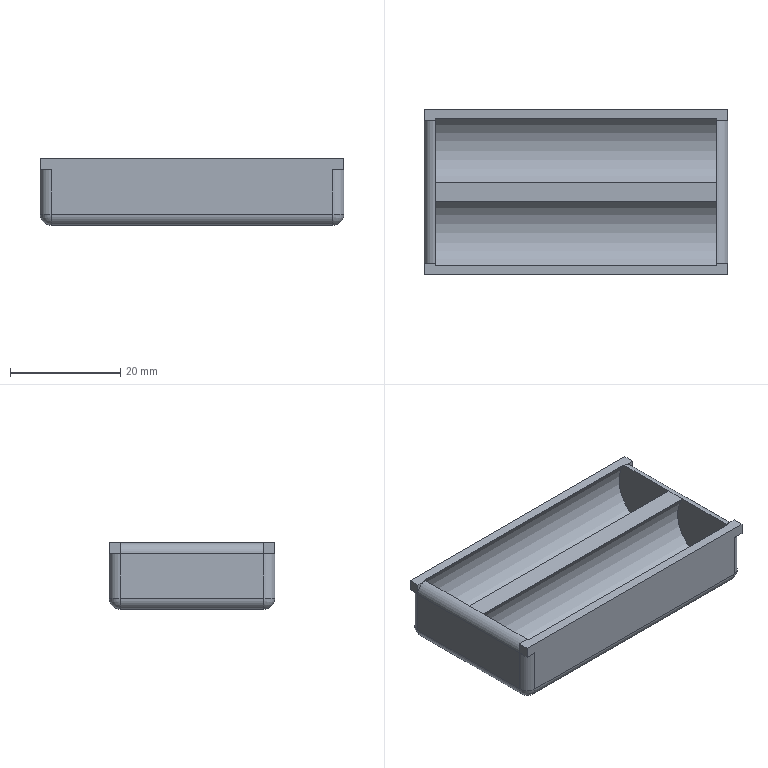Part | NX | features DATUM_CSYS 3, EXTRUDE 2, SKETCH 2, BLEND 1 | 1 solid | 40 faces | box 55 x 30 x 12 mm | volume 6346 mm3 | plane 24 | cylinder 12 | sphere 4 | commonest cylinder face diameters 4 x10 14 x2
STEP:
#1=CARTESIAN_POINT('',(-27.5,-13.,12.));
#2=VERTEX_POINT('',#1);
#3=CARTESIAN_POINT('',(-27.5,-15.,12.));
#4=VERTEX_POINT('',#3);
#5=CARTESIAN_POINT('',(-27.5,15.,12.));
#6=DIRECTION('',(0.,-1.,0.));
#7=VECTOR('',#6,1000.);
#8=LINE('',#5,#7);
#9=EDGE_CURVE('',#2,#4,#8,.T.);
#10=ORIENTED_EDGE('',*,*,#9,.F.);
#11=CARTESIAN_POINT('',(-27.5,-13.,10.));
#12=VERTEX_POINT('',#11);
#13=CARTESIAN_POINT('',(-27.5,-13.,12.));
#14=DIRECTION('',(0.,0.,-1.));
#15=VECTOR('',#14,1000.);
#16=LINE('',#13,#15);
#17=EDGE_CURVE('',#2,#12,#16,.T.);
#18=ORIENTED_EDGE('',*,*,#17,.T.);
#19=CARTESIAN_POINT('',(-27.5,-15.,10.));
#20=VERTEX_POINT('',#19);
#21=CARTESIAN_POINT('',(-27.5,-13.,10.));
#22=DIRECTION('',(0.,-1.,0.));
#23=VECTOR('',#22,1000.);
#24=LINE('',#21,#23);
#25=EDGE_CURVE('',#12,#20,#24,.T.);
#26=ORIENTED_EDGE('',*,*,#25,.T.);
#27=CARTESIAN_POINT('',(-27.5,-15.,12.));
#28=DIRECTION('',(0.,0.,-1.));
#29=VECTOR('',#28,1000.);
#30=LINE('',#27,#29);
#31=EDGE_CURVE('',#4,#20,#30,.T.);
#32=ORIENTED_EDGE('',*,*,#31,.F.);
#33=EDGE_LOOP('',(#10,#18,#26,#32));
#34=FACE_BOUND('',#33,.T.);
#35=CARTESIAN_POINT('',(-27.5,15.,12.));
#36=DIRECTION('',(1.,0.,0.));
#37=DIRECTION('',(0.,1.,0.));
#38=AXIS2_PLACEMENT_3D('',#35,#36,#37);
#39=PLANE('',#38);
#40=ADVANCED_FACE('',(#34),#39,.F.);
#41=CARTESIAN_POINT('',(-27.5,15.,10.));
#42=VERTEX_POINT('',#41);
#43=CARTESIAN_POINT('',(-27.5,13.,10.));
#44=VERTEX_POINT('',#43);
#45=CARTESIAN_POINT('',(-27.5,13.,10.));
#46=DIRECTION('',(0.,-1.,0.));
#47=VECTOR('',#46,1000.);
#48=LINE('',#45,#47);
#49=EDGE_CURVE('',#42,#44,#48,.T.);
#50=ORIENTED_EDGE('',*,*,#49,.T.);
#51=CARTESIAN_POINT('',(-27.5,13.,12.));
#52=VERTEX_POINT('',#51);
#53=CARTESIAN_POINT('',(-27.5,13.,12.));
#54=DIRECTION('',(0.,0.,1.));
#55=VECTOR('',#54,1000.);
#56=LINE('',#53,#55);
#57=EDGE_CURVE('',#44,#52,#56,.T.);
#58=ORIENTED_EDGE('',*,*,#57,.T.);
#59=CARTESIAN_POINT('',(-27.5,15.,12.));
#60=VERTEX_POINT('',#59);
#61=CARTESIAN_POINT('',(-27.5,15.,12.));
#62=DIRECTION('',(0.,-1.,0.));
#63=VECTOR('',#62,1000.);
#64=LINE('',#61,#63);
#65=EDGE_CURVE('',#60,#52,#64,.T.);
#66=ORIENTED_EDGE('',*,*,#65,.F.);
#67=CARTESIAN_POINT('',(-27.5,15.,12.));
#68=DIRECTION('',(0.,0.,-1.));
#69=VECTOR('',#68,1000.);
#70=LINE('',#67,#69);
#71=EDGE_CURVE('',#60,#42,#70,.T.);
#72=ORIENTED_EDGE('',*,*,#71,.T.);
#73=EDGE_LOOP('',(#50,#58,#66,#72));
#74=FACE_BOUND('',#73,.T.);
#75=CARTESIAN_POINT('',(-27.5,15.,12.));
#76=DIRECTION('',(1.,0.,0.));
#77=DIRECTION('',(0.,1.,0.));
#78=AXIS2_PLACEMENT_3D('',#75,#76,#77);
#79=PLANE('',#78);
#80=ADVANCED_FACE('',(#74),#79,.F.);
#81=CARTESIAN_POINT('',(27.5,13.,12.));
#82=VERTEX_POINT('',#81);
#83=CARTESIAN_POINT('',(27.5,15.,12.));
#84=VERTEX_POINT('',#83);
#85=CARTESIAN_POINT('',(27.5,-15.,12.));
#86=DIRECTION('',(0.,1.,0.));
#87=VECTOR('',#86,1000.);
#88=LINE('',#85,#87);
#89=EDGE_CURVE('',#82,#84,#88,.T.);
#90=ORIENTED_EDGE('',*,*,#89,.F.);
#91=CARTESIAN_POINT('',(27.5,13.,10.));
#92=VERTEX_POINT('',#91);
#93=CARTESIAN_POINT('',(27.5,13.,12.));
#94=DIRECTION('',(0.,0.,-1.));
#95=VECTOR('',#94,1000.);
#96=LINE('',#93,#95);
#97=EDGE_CURVE('',#82,#92,#96,.T.);
#98=ORIENTED_EDGE('',*,*,#97,.T.);
#99=CARTESIAN_POINT('',(27.5,15.,10.));
#100=VERTEX_POINT('',#99);
#101=CARTESIAN_POINT('',(27.5,13.,10.));
#102=DIRECTION('',(0.,1.,0.));
#103=VECTOR('',#102,1000.);
#104=LINE('',#101,#103);
#105=EDGE_CURVE('',#92,#100,#104,.T.);
#106=ORIENTED_EDGE('',*,*,#105,.T.);
#107=CARTESIAN_POINT('',(27.5,15.,12.));
#108=DIRECTION('',(0.,0.,-1.));
#109=VECTOR('',#108,1000.);
#110=LINE('',#107,#109);
#111=EDGE_CURVE('',#84,#100,#110,.T.);
#112=ORIENTED_EDGE('',*,*,#111,.F.);
#113=EDGE_LOOP('',(#90,#98,#106,#112));
#114=FACE_BOUND('',#113,.T.);
#115=CARTESIAN_POINT('',(27.5,-15.,12.));
#116=DIRECTION('',(-1.,0.,0.));
#117=DIRECTION('',(0.,-1.,0.));
#118=AXIS2_PLACEMENT_3D('',#115,#116,#117);
#119=PLANE('',#118);
#120=ADVANCED_FACE('',(#114),#119,.F.);
#121=CARTESIAN_POINT('',(27.5,-15.,10.));
#122=VERTEX_POINT('',#121);
#123=CARTESIAN_POINT('',(27.5,-13.,10.));
#124=VERTEX_POINT('',#123);
#125=CARTESIAN_POINT('',(27.5,-13.,10.));
#126=DIRECTION('',(0.,1.,0.));
#127=VECTOR('',#126,1000.);
#128=LINE('',#125,#127);
#129=EDGE_CURVE('',#122,#124,#128,.T.);
#130=ORIENTED_EDGE('',*,*,#129,.T.);
#131=CARTESIAN_POINT('',(27.5,-13.,12.));
#132=VERTEX_POINT('',#131);
#133=CARTESIAN_POINT('',(27.5,-13.,12.));
#134=DIRECTION('',(0.,0.,1.));
#135=VECTOR('',#134,1000.);
#136=LINE('',#133,#135);
#137=EDGE_CURVE('',#124,#132,#136,.T.);
#138=ORIENTED_EDGE('',*,*,#137,.T.);
#139=CARTESIAN_POINT('',(27.5,-15.,12.));
#140=VERTEX_POINT('',#139);
#141=CARTESIAN_POINT('',(27.5,-15.,12.));
#142=DIRECTION('',(0.,1.,0.));
#143=VECTOR('',#142,1000.);
#144=LINE('',#141,#143);
#145=EDGE_CURVE('',#140,#132,#144,.T.);
#146=ORIENTED_EDGE('',*,*,#145,.F.);
#147=CARTESIAN_POINT('',(27.5,-15.,12.));
#148=DIRECTION('',(0.,0.,-1.));
#149=VECTOR('',#148,1000.);
#150=LINE('',#147,#149);
#151=EDGE_CURVE('',#140,#122,#150,.T.);
#152=ORIENTED_EDGE('',*,*,#151,.T.);
#153=EDGE_LOOP('',(#130,#138,#146,#152));
#154=FACE_BOUND('',#153,.T.);
#155=CARTESIAN_POINT('',(27.5,-15.,12.));
#156=DIRECTION('',(-1.,0.,0.));
#157=DIRECTION('',(0.,-1.,0.));
#158=AXIS2_PLACEMENT_3D('',#155,#156,#157);
#159=PLANE('',#158);
#160=ADVANCED_FACE('',(#154),#159,.F.);
#161=ORIENTED_EDGE('',*,*,#145,.T.);
#162=CARTESIAN_POINT('',(25.5,-13.,12.));
#163=VERTEX_POINT('',#162);
#164=CARTESIAN_POINT('',(25.5,-13.,12.));
#165=DIRECTION('',(-1.,0.,0.));
#166=VECTOR('',#165,1000.);
#167=LINE('',#164,#166);
#168=EDGE_CURVE('',#132,#163,#167,.T.);
#169=ORIENTED_EDGE('',*,*,#168,.T.);
#170=CARTESIAN_POINT('',(25.5,-13.245,12.));
#171=VERTEX_POINT('',#170);
#172=CARTESIAN_POINT('',(25.5,0.,12.));
#173=DIRECTION('',(0.,-1.,0.));
#174=VECTOR('',#173,1000.);
#175=LINE('',#172,#174);
#176=EDGE_CURVE('',#163,#171,#175,.T.);
#177=ORIENTED_EDGE('',*,*,#176,.T.);
#178=CARTESIAN_POINT('',(-25.5,-13.245,12.));
#179=VERTEX_POINT('',#178);
#180=CARTESIAN_POINT('',(25.5,-13.245,12.));
#181=DIRECTION('',(-1.,0.,0.));
#182=VECTOR('',#181,1000.);
#183=LINE('',#180,#182);
#184=EDGE_CURVE('',#179,#171,#183,.F.);
#185=ORIENTED_EDGE('',*,*,#184,.F.);
#186=CARTESIAN_POINT('',(-25.5,-13.,12.));
#187=VERTEX_POINT('',#186);
#188=CARTESIAN_POINT('',(-25.5,0.,12.));
#189=DIRECTION('',(0.,-1.,0.));
#190=VECTOR('',#189,1000.);
#191=LINE('',#188,#190);
#192=EDGE_CURVE('',#187,#179,#191,.T.);
#193=ORIENTED_EDGE('',*,*,#192,.F.);
#194=CARTESIAN_POINT('',(-25.5,-13.,12.));
#195=DIRECTION('',(-1.,0.,0.));
#196=VECTOR('',#195,1000.);
#197=LINE('',#194,#196);
#198=EDGE_CURVE('',#187,#2,#197,.T.);
#199=ORIENTED_EDGE('',*,*,#198,.T.);
#200=ORIENTED_EDGE('',*,*,#9,.T.);
#201=CARTESIAN_POINT('',(-27.5,-15.,12.));
#202=DIRECTION('',(1.,0.,0.));
#203=VECTOR('',#202,1000.);
#204=LINE('',#201,#203);
#205=EDGE_CURVE('',#4,#140,#204,.T.);
#206=ORIENTED_EDGE('',*,*,#205,.T.);
#207=EDGE_LOOP('',(#161,#169,#177,#185,#193,#199,#200,#206));
#208=FACE_BOUND('',#207,.T.);
#209=CARTESIAN_POINT('',(0.,0.,12.));
#210=DIRECTION('',(0.,0.,1.));
#211=DIRECTION('',(1.,0.,0.));
#212=AXIS2_PLACEMENT_3D('',#209,#210,#211);
#213=PLANE('',#212);
#214=ADVANCED_FACE('',(#208),#213,.T.);
#215=CARTESIAN_POINT('',(25.5,-1.755,12.));
#216=VERTEX_POINT('',#215);
#217=CARTESIAN_POINT('',(-25.5,-1.755,12.));
#218=VERTEX_POINT('',#217);
#219=CARTESIAN_POINT('',(25.5,-1.755,12.));
#220=DIRECTION('',(-1.,0.,0.));
#221=VECTOR('',#220,1000.);
#222=LINE('',#219,#221);
#223=EDGE_CURVE('',#216,#218,#222,.T.);
#224=ORIENTED_EDGE('',*,*,#223,.F.);
#225=CARTESIAN_POINT('',(25.5,1.755,12.));
#226=VERTEX_POINT('',#225);
#227=CARTESIAN_POINT('',(25.5,15.,12.));
#228=DIRECTION('',(0.,1.,0.));
#229=VECTOR('',#228,1000.);
#230=LINE('',#227,#229);
#231=EDGE_CURVE('',#216,#226,#230,.T.);
#232=ORIENTED_EDGE('',*,*,#231,.T.);
#233=CARTESIAN_POINT('',(-25.5,1.755,12.));
#234=VERTEX_POINT('',#233);
#235=CARTESIAN_POINT('',(25.5,1.755,12.));
#236=DIRECTION('',(-1.,0.,0.));
#237=VECTOR('',#236,1000.);
#238=LINE('',#235,#237);
#239=EDGE_CURVE('',#234,#226,#238,.F.);
#240=ORIENTED_EDGE('',*,*,#239,.F.);
#241=CARTESIAN_POINT('',(-25.5,-15.,12.));
#242=DIRECTION('',(0.,-1.,0.));
#243=VECTOR('',#242,1000.);
#244=LINE('',#241,#243);
#245=EDGE_CURVE('',#234,#218,#244,.T.);
#246=ORIENTED_EDGE('',*,*,#245,.T.);
#247=EDGE_LOOP('',(#224,#232,#240,#246));
#248=FACE_BOUND('',#247,.T.);
#249=CARTESIAN_POINT('',(0.,0.,12.));
#250=DIRECTION('',(0.,0.,1.));
#251=DIRECTION('',(1.,0.,0.));
#252=AXIS2_PLACEMENT_3D('',#249,#250,#251);
#253=PLANE('',#252);
#254=ADVANCED_FACE('',(#248),#253,.T.);
#255=CARTESIAN_POINT('',(25.5,13.245,12.));
#256=VERTEX_POINT('',#255);
#257=CARTESIAN_POINT('',(25.5,13.,12.));
#258=VERTEX_POINT('',#257);
#259=CARTESIAN_POINT('',(25.5,0.,12.));
#260=DIRECTION('',(0.,-1.,0.));
#261=VECTOR('',#260,1000.);
#262=LINE('',#259,#261);
#263=EDGE_CURVE('',#256,#258,#262,.T.);
#264=ORIENTED_EDGE('',*,*,#263,.T.);
#265=CARTESIAN_POINT('',(25.5,13.,12.));
#266=DIRECTION('',(1.,0.,0.));
#267=VECTOR('',#266,1000.);
#268=LINE('',#265,#267);
#269=EDGE_CURVE('',#258,#82,#268,.T.);
#270=ORIENTED_EDGE('',*,*,#269,.T.);
#271=ORIENTED_EDGE('',*,*,#89,.T.);
#272=CARTESIAN_POINT('',(27.5,15.,12.));
#273=DIRECTION('',(-1.,0.,0.));
#274=VECTOR('',#273,1000.);
#275=LINE('',#272,#274);
#276=EDGE_CURVE('',#84,#60,#275,.T.);
#277=ORIENTED_EDGE('',*,*,#276,.T.);
#278=ORIENTED_EDGE('',*,*,#65,.T.);
#279=CARTESIAN_POINT('',(-25.5,13.,12.));
#280=VERTEX_POINT('',#279);
#281=CARTESIAN_POINT('',(-25.5,13.,12.));
#282=DIRECTION('',(1.,0.,0.));
#283=VECTOR('',#282,1000.);
#284=LINE('',#281,#283);
#285=EDGE_CURVE('',#52,#280,#284,.T.);
#286=ORIENTED_EDGE('',*,*,#285,.T.);
#287=CARTESIAN_POINT('',(-25.5,13.245,12.));
#288=VERTEX_POINT('',#287);
#289=CARTESIAN_POINT('',(-25.5,0.,12.));
#290=DIRECTION('',(0.,-1.,0.));
#291=VECTOR('',#290,1000.);
#292=LINE('',#289,#291);
#293=EDGE_CURVE('',#288,#280,#292,.T.);
#294=ORIENTED_EDGE('',*,*,#293,.F.);
#295=CARTESIAN_POINT('',(25.5,13.245,12.));
#296=DIRECTION('',(-1.,0.,0.));
#297=VECTOR('',#296,1000.);
#298=LINE('',#295,#297);
#299=EDGE_CURVE('',#256,#288,#298,.T.);
#300=ORIENTED_EDGE('',*,*,#299,.F.);
#301=EDGE_LOOP('',(#264,#270,#271,#277,#278,#286,#294,#300));
#302=FACE_BOUND('',#301,.T.);
#303=CARTESIAN_POINT('',(0.,0.,12.));
#304=DIRECTION('',(0.,0.,1.));
#305=DIRECTION('',(1.,0.,0.));
#306=AXIS2_PLACEMENT_3D('',#303,#304,#305);
#307=PLANE('',#306);
#308=ADVANCED_FACE('',(#302),#307,.T.);
#309=CARTESIAN_POINT('',(-27.5,-13.,2.));
#310=VERTEX_POINT('',#309);
#311=CARTESIAN_POINT('',(-27.5,-13.,12.));
#312=DIRECTION('',(0.,0.,-1.));
#313=VECTOR('',#312,1000.);
#314=LINE('',#311,#313);
#315=EDGE_CURVE('',#310,#12,#314,.F.);
#316=ORIENTED_EDGE('',*,*,#315,.T.);
#317=CARTESIAN_POINT('',(-27.5,15.,10.));
#318=DIRECTION('',(0.,-1.,0.));
#319=VECTOR('',#318,1000.);
#320=LINE('',#317,#319);
#321=EDGE_CURVE('',#12,#44,#320,.F.);
#322=ORIENTED_EDGE('',*,*,#321,.T.);
#323=CARTESIAN_POINT('',(-27.5,13.,2.));
#324=VERTEX_POINT('',#323);
#325=CARTESIAN_POINT('',(-27.5,13.,12.));
#326=DIRECTION('',(0.,0.,-1.));
#327=VECTOR('',#326,1000.);
#328=LINE('',#325,#327);
#329=EDGE_CURVE('',#44,#324,#328,.T.);
#330=ORIENTED_EDGE('',*,*,#329,.T.);
#331=CARTESIAN_POINT('',(-27.5,15.,2.));
#332=DIRECTION('',(0.,-1.,0.));
#333=VECTOR('',#332,1000.);
#334=LINE('',#331,#333);
#335=EDGE_CURVE('',#324,#310,#334,.T.);
#336=ORIENTED_EDGE('',*,*,#335,.T.);
#337=EDGE_LOOP('',(#316,#322,#330,#336));
#338=FACE_BOUND('',#337,.T.);
#339=CARTESIAN_POINT('',(-27.5,15.,12.));
#340=DIRECTION('',(1.,0.,0.));
#341=DIRECTION('',(0.,1.,0.));
#342=AXIS2_PLACEMENT_3D('',#339,#340,#341);
#343=PLANE('',#342);
#344=ADVANCED_FACE('',(#338),#343,.F.);
#345=CARTESIAN_POINT('',(25.5,-15.,2.));
#346=VERTEX_POINT('',#345);
#347=CARTESIAN_POINT('',(25.5,-15.,10.));
#348=VERTEX_POINT('',#347);
#349=CARTESIAN_POINT('',(25.5,-15.,12.));
#350=DIRECTION('',(0.,0.,-1.));
#351=VECTOR('',#350,1000.);
#352=LINE('',#349,#351);
#353=EDGE_CURVE('',#346,#348,#352,.F.);
#354=ORIENTED_EDGE('',*,*,#353,.T.);
#355=CARTESIAN_POINT('',(25.5,-15.,10.));
#356=DIRECTION('',(1.,0.,0.));
#357=VECTOR('',#356,1000.);
#358=LINE('',#355,#357);
#359=EDGE_CURVE('',#348,#122,#358,.T.);
#360=ORIENTED_EDGE('',*,*,#359,.T.);
#361=ORIENTED_EDGE('',*,*,#151,.F.);
#362=ORIENTED_EDGE('',*,*,#205,.F.);
#363=ORIENTED_EDGE('',*,*,#31,.T.);
#364=CARTESIAN_POINT('',(-25.5,-15.,10.));
#365=VERTEX_POINT('',#364);
#366=CARTESIAN_POINT('',(-25.5,-15.,10.));
#367=DIRECTION('',(1.,0.,0.));
#368=VECTOR('',#367,1000.);
#369=LINE('',#366,#368);
#370=EDGE_CURVE('',#20,#365,#369,.T.);
#371=ORIENTED_EDGE('',*,*,#370,.T.);
#372=CARTESIAN_POINT('',(-25.5,-15.,2.));
#373=VERTEX_POINT('',#372);
#374=CARTESIAN_POINT('',(-25.5,-15.,12.));
#375=DIRECTION('',(0.,0.,-1.));
#376=VECTOR('',#375,1000.);
#377=LINE('',#374,#376);
#378=EDGE_CURVE('',#365,#373,#377,.T.);
#379=ORIENTED_EDGE('',*,*,#378,.T.);
#380=CARTESIAN_POINT('',(-27.5,-15.,2.));
#381=DIRECTION('',(1.,0.,0.));
#382=VECTOR('',#381,1000.);
#383=LINE('',#380,#382);
#384=EDGE_CURVE('',#373,#346,#383,.T.);
#385=ORIENTED_EDGE('',*,*,#384,.T.);
#386=EDGE_LOOP('',(#354,#360,#361,#362,#363,#371,#379,#385));
#387=FACE_BOUND('',#386,.T.);
#388=CARTESIAN_POINT('',(-27.5,-15.,12.));
#389=DIRECTION('',(0.,1.,0.));
#390=DIRECTION('',(0.,0.,1.));
#391=AXIS2_PLACEMENT_3D('',#388,#389,#390);
#392=PLANE('',#391);
#393=ADVANCED_FACE('',(#387),#392,.F.);
#394=CARTESIAN_POINT('',(27.5,13.,2.));
#395=VERTEX_POINT('',#394);
#396=CARTESIAN_POINT('',(27.5,13.,12.));
#397=DIRECTION('',(0.,0.,-1.));
#398=VECTOR('',#397,1000.);
#399=LINE('',#396,#398);
#400=EDGE_CURVE('',#395,#92,#399,.F.);
#401=ORIENTED_EDGE('',*,*,#400,.T.);
#402=CARTESIAN_POINT('',(27.5,-15.,10.));
#403=DIRECTION('',(0.,1.,0.));
#404=VECTOR('',#403,1000.);
#405=LINE('',#402,#404);
#406=EDGE_CURVE('',#92,#124,#405,.F.);
#407=ORIENTED_EDGE('',*,*,#406,.T.);
#408=CARTESIAN_POINT('',(27.5,-13.,2.));
#409=VERTEX_POINT('',#408);
#410=CARTESIAN_POINT('',(27.5,-13.,12.));
#411=DIRECTION('',(0.,0.,-1.));
#412=VECTOR('',#411,1000.);
#413=LINE('',#410,#412);
#414=EDGE_CURVE('',#124,#409,#413,.T.);
#415=ORIENTED_EDGE('',*,*,#414,.T.);
#416=CARTESIAN_POINT('',(27.5,-15.,2.));
#417=DIRECTION('',(0.,1.,0.));
#418=VECTOR('',#417,1000.);
#419=LINE('',#416,#418);
#420=EDGE_CURVE('',#409,#395,#419,.T.);
#421=ORIENTED_EDGE('',*,*,#420,.T.);
#422=EDGE_LOOP('',(#401,#407,#415,#421));
#423=FACE_BOUND('',#422,.T.);
#424=CARTESIAN_POINT('',(27.5,-15.,12.));
#425=DIRECTION('',(-1.,0.,0.));
#426=DIRECTION('',(0.,-1.,0.));
#427=AXIS2_PLACEMENT_3D('',#424,#425,#426);
#428=PLANE('',#427);
#429=ADVANCED_FACE('',(#423),#428,.F.);
#430=ORIENTED_EDGE('',*,*,#111,.T.);
#431=CARTESIAN_POINT('',(25.5,15.,10.));
#432=VERTEX_POINT('',#431);
#433=CARTESIAN_POINT('',(25.5,15.,10.));
#434=DIRECTION('',(-1.,0.,0.));
#435=VECTOR('',#434,1000.);
#436=LINE('',#433,#435);
#437=EDGE_CURVE('',#100,#432,#436,.T.);
#438=ORIENTED_EDGE('',*,*,#437,.T.);
#439=CARTESIAN_POINT('',(25.5,15.,2.));
#440=VERTEX_POINT('',#439);
#441=CARTESIAN_POINT('',(25.5,15.,12.));
#442=DIRECTION('',(0.,0.,-1.));
#443=VECTOR('',#442,1000.);
#444=LINE('',#441,#443);
#445=EDGE_CURVE('',#432,#440,#444,.T.);
#446=ORIENTED_EDGE('',*,*,#445,.T.);
#447=CARTESIAN_POINT('',(-25.5,15.,2.));
#448=VERTEX_POINT('',#447);
#449=CARTESIAN_POINT('',(27.5,15.,2.));
#450=DIRECTION('',(-1.,0.,0.));
#451=VECTOR('',#450,1000.);
#452=LINE('',#449,#451);
#453=EDGE_CURVE('',#440,#448,#452,.T.);
#454=ORIENTED_EDGE('',*,*,#453,.T.);
#455=CARTESIAN_POINT('',(-25.5,15.,10.));
#456=VERTEX_POINT('',#455);
#457=CARTESIAN_POINT('',(-25.5,15.,12.));
#458=DIRECTION('',(0.,0.,-1.));
#459=VECTOR('',#458,1000.);
#460=LINE('',#457,#459);
#461=EDGE_CURVE('',#448,#456,#460,.F.);
#462=ORIENTED_EDGE('',*,*,#461,.T.);
#463=CARTESIAN_POINT('',(-25.5,15.,10.));
#464=DIRECTION('',(-1.,0.,0.));
#465=VECTOR('',#464,1000.);
#466=LINE('',#463,#465);
#467=EDGE_CURVE('',#456,#42,#466,.T.);
#468=ORIENTED_EDGE('',*,*,#467,.T.);
#469=ORIENTED_EDGE('',*,*,#71,.F.);
#470=ORIENTED_EDGE('',*,*,#276,.F.);
#471=EDGE_LOOP('',(#430,#438,#446,#454,#462,#468,#469,#470));
#472=FACE_BOUND('',#471,.T.);
#473=CARTESIAN_POINT('',(27.5,15.,12.));
#474=DIRECTION('',(0.,-1.,0.));
#475=DIRECTION('',(1.,0.,0.));
#476=AXIS2_PLACEMENT_3D('',#473,#474,#475);
#477=PLANE('',#476);
#478=ADVANCED_FACE('',(#472),#477,.F.);
#479=CARTESIAN_POINT('',(25.5,-13.,0.));
#480=VERTEX_POINT('',#479);
#481=CARTESIAN_POINT('',(-25.5,-13.,0.));
#482=VERTEX_POINT('',#481);
#483=CARTESIAN_POINT('',(0.,-13.,0.));
#484=DIRECTION('',(1.,0.,0.));
#485=VECTOR('',#484,1000.);
#486=LINE('',#483,#485);
#487=EDGE_CURVE('',#480,#482,#486,.F.);
#488=ORIENTED_EDGE('',*,*,#487,.T.);
#489=CARTESIAN_POINT('',(-25.5,13.,0.));
#490=VERTEX_POINT('',#489);
#491=CARTESIAN_POINT('',(-25.5,0.,0.));
#492=DIRECTION('',(0.,-1.,0.));
#493=VECTOR('',#492,1000.);
#494=LINE('',#491,#493);
#495=EDGE_CURVE('',#482,#490,#494,.F.);
#496=ORIENTED_EDGE('',*,*,#495,.T.);
#497=CARTESIAN_POINT('',(25.5,13.,0.));
#498=VERTEX_POINT('',#497);
#499=CARTESIAN_POINT('',(0.,13.,0.));
#500=DIRECTION('',(-1.,0.,0.));
#501=VECTOR('',#500,1000.);
#502=LINE('',#499,#501);
#503=EDGE_CURVE('',#490,#498,#502,.F.);
#504=ORIENTED_EDGE('',*,*,#503,.T.);
#505=CARTESIAN_POINT('',(25.5,0.,0.));
#506=DIRECTION('',(0.,1.,0.));
#507=VECTOR('',#506,1000.);
#508=LINE('',#505,#507);
#509=EDGE_CURVE('',#498,#480,#508,.F.);
#510=ORIENTED_EDGE('',*,*,#509,.T.);
#511=EDGE_LOOP('',(#488,#496,#504,#510));
#512=FACE_BOUND('',#511,.T.);
#513=CARTESIAN_POINT('',(0.,0.,0.));
#514=DIRECTION('',(0.,0.,1.));
#515=DIRECTION('',(1.,0.,0.));
#516=AXIS2_PLACEMENT_3D('',#513,#514,#515);
#517=PLANE('',#516);
#518=ADVANCED_FACE('',(#512),#517,.F.);
#519=ORIENTED_EDGE('',*,*,#299,.T.);
#520=CARTESIAN_POINT('',(-25.5,7.5,8.));
#521=DIRECTION('',(-1.,0.,0.));
#522=DIRECTION('',(0.,1.,0.));
#523=AXIS2_PLACEMENT_3D('',#520,#521,#522);
#524=CIRCLE('',#523,7.);
#525=EDGE_CURVE('',#234,#288,#524,.F.);
#526=ORIENTED_EDGE('',*,*,#525,.F.);
#527=ORIENTED_EDGE('',*,*,#239,.T.);
#528=CARTESIAN_POINT('',(25.5,7.5,8.));
#529=DIRECTION('',(-1.,0.,0.));
#530=DIRECTION('',(0.,1.,0.));
#531=AXIS2_PLACEMENT_3D('',#528,#529,#530);
#532=CIRCLE('',#531,7.);
#533=EDGE_CURVE('',#226,#256,#532,.F.);
#534=ORIENTED_EDGE('',*,*,#533,.T.);
#535=EDGE_LOOP('',(#519,#526,#527,#534));
#536=FACE_BOUND('',#535,.T.);
#537=CARTESIAN_POINT('',(25.5,7.5,8.));
#538=DIRECTION('',(-1.,0.,0.));
#539=DIRECTION('',(0.,0.,1.));
#540=AXIS2_PLACEMENT_3D('',#537,#538,#539);
#541=CYLINDRICAL_SURFACE('',#540,7.);
#542=ADVANCED_FACE('',(#536),#541,.F.);
#543=ORIENTED_EDGE('',*,*,#533,.F.);
#544=CARTESIAN_POINT('',(25.5,0.,12.));
#545=DIRECTION('',(0.,-1.,0.));
#546=VECTOR('',#545,1000.);
#547=LINE('',#544,#546);
#548=EDGE_CURVE('',#258,#226,#547,.T.);
#549=ORIENTED_EDGE('',*,*,#548,.F.);
#550=ORIENTED_EDGE('',*,*,#263,.F.);
#551=EDGE_LOOP('',(#543,#549,#550));
#552=FACE_BOUND('',#551,.T.);
#553=CARTESIAN_POINT('',(25.5,7.5,8.));
#554=DIRECTION('',(-1.,0.,0.));
#555=DIRECTION('',(0.,0.,1.));
#556=AXIS2_PLACEMENT_3D('',#553,#554,#555);
#557=PLANE('',#556);
#558=ADVANCED_FACE('',(#552),#557,.T.);
#559=ORIENTED_EDGE('',*,*,#293,.T.);
#560=CARTESIAN_POINT('',(-25.5,0.,12.));
#561=DIRECTION('',(0.,-1.,0.));
#562=VECTOR('',#561,1000.);
#563=LINE('',#560,#562);
#564=EDGE_CURVE('',#280,#234,#563,.T.);
#565=ORIENTED_EDGE('',*,*,#564,.T.);
#566=ORIENTED_EDGE('',*,*,#525,.T.);
#567=EDGE_LOOP('',(#559,#565,#566));
#568=FACE_BOUND('',#567,.T.);
#569=CARTESIAN_POINT('',(-25.5,7.5,8.));
#570=DIRECTION('',(-1.,0.,0.));
#571=DIRECTION('',(0.,0.,1.));
#572=AXIS2_PLACEMENT_3D('',#569,#570,#571);
#573=PLANE('',#572);
#574=ADVANCED_FACE('',(#568),#573,.F.);
#575=ORIENTED_EDGE('',*,*,#223,.T.);
#576=CARTESIAN_POINT('',(-25.5,-7.5,8.));
#577=DIRECTION('',(-1.,0.,0.));
#578=DIRECTION('',(0.,1.,0.));
#579=AXIS2_PLACEMENT_3D('',#576,#577,#578);
#580=CIRCLE('',#579,7.);
#581=EDGE_CURVE('',#179,#218,#580,.F.);
#582=ORIENTED_EDGE('',*,*,#581,.F.);
#583=ORIENTED_EDGE('',*,*,#184,.T.);
#584=CARTESIAN_POINT('',(25.5,-7.5,8.));
#585=DIRECTION('',(-1.,0.,0.));
#586=DIRECTION('',(0.,1.,0.));
#587=AXIS2_PLACEMENT_3D('',#584,#585,#586);
#588=CIRCLE('',#587,7.);
#589=EDGE_CURVE('',#171,#216,#588,.F.);
#590=ORIENTED_EDGE('',*,*,#589,.T.);
#591=EDGE_LOOP('',(#575,#582,#583,#590));
#592=FACE_BOUND('',#591,.T.);
#593=CARTESIAN_POINT('',(25.5,-7.5,8.));
#594=DIRECTION('',(-1.,0.,0.));
#595=DIRECTION('',(0.,0.,1.));
#596=AXIS2_PLACEMENT_3D('',#593,#594,#595);
#597=CYLINDRICAL_SURFACE('',#596,7.);
#598=ADVANCED_FACE('',(#592),#597,.F.);
#599=ORIENTED_EDGE('',*,*,#589,.F.);
#600=ORIENTED_EDGE('',*,*,#176,.F.);
#601=CARTESIAN_POINT('',(25.5,0.,12.));
#602=DIRECTION('',(0.,-1.,0.));
#603=VECTOR('',#602,1000.);
#604=LINE('',#601,#603);
#605=EDGE_CURVE('',#216,#163,#604,.T.);
#606=ORIENTED_EDGE('',*,*,#605,.F.);
#607=EDGE_LOOP('',(#599,#600,#606));
#608=FACE_BOUND('',#607,.T.);
#609=CARTESIAN_POINT('',(25.5,-7.5,8.));
#610=DIRECTION('',(-1.,0.,0.));
#611=DIRECTION('',(0.,0.,1.));
#612=AXIS2_PLACEMENT_3D('',#609,#610,#611);
#613=PLANE('',#612);
#614=ADVANCED_FACE('',(#608),#613,.T.);
#615=CARTESIAN_POINT('',(-25.5,0.,12.));
#616=DIRECTION('',(0.,-1.,0.));
#617=VECTOR('',#616,1000.);
#618=LINE('',#615,#617);
#619=EDGE_CURVE('',#218,#187,#618,.T.);
#620=ORIENTED_EDGE('',*,*,#619,.T.);
#621=ORIENTED_EDGE('',*,*,#192,.T.);
#622=ORIENTED_EDGE('',*,*,#581,.T.);
#623=EDGE_LOOP('',(#620,#621,#622));
#624=FACE_BOUND('',#623,.T.);
#625=CARTESIAN_POINT('',(-25.5,-7.5,8.));
#626=DIRECTION('',(-1.,0.,0.));
#627=DIRECTION('',(0.,0.,1.));
#628=AXIS2_PLACEMENT_3D('',#625,#626,#627);
#629=PLANE('',#628);
#630=ADVANCED_FACE('',(#624),#629,.F.);
#631=ORIENTED_EDGE('',*,*,#437,.F.);
#632=ORIENTED_EDGE('',*,*,#105,.F.);
#633=CARTESIAN_POINT('',(25.5,13.,10.));
#634=DIRECTION('',(0.,0.,1.));
#635=DIRECTION('',(1.,0.,0.));
#636=AXIS2_PLACEMENT_3D('',#633,#634,#635);
#637=CIRCLE('',#636,2.);
#638=EDGE_CURVE('',#432,#92,#637,.F.);
#639=ORIENTED_EDGE('',*,*,#638,.F.);
#640=EDGE_LOOP('',(#631,#632,#639));
#641=FACE_BOUND('',#640,.T.);
#642=CARTESIAN_POINT('',(25.5,13.,10.));
#643=DIRECTION('',(0.,0.,-1.));
#644=DIRECTION('',(-1.,0.,0.));
#645=AXIS2_PLACEMENT_3D('',#642,#643,#644);
#646=PLANE('',#645);
#647=ADVANCED_FACE('',(#641),#646,.T.);
#648=ORIENTED_EDGE('',*,*,#129,.F.);
#649=ORIENTED_EDGE('',*,*,#359,.F.);
#650=CARTESIAN_POINT('',(25.5,-13.,10.));
#651=DIRECTION('',(0.,0.,1.));
#652=DIRECTION('',(1.,0.,0.));
#653=AXIS2_PLACEMENT_3D('',#650,#651,#652);
#654=CIRCLE('',#653,2.);
#655=EDGE_CURVE('',#124,#348,#654,.F.);
#656=ORIENTED_EDGE('',*,*,#655,.F.);
#657=EDGE_LOOP('',(#648,#649,#656));
#658=FACE_BOUND('',#657,.T.);
#659=CARTESIAN_POINT('',(25.5,-13.,10.));
#660=DIRECTION('',(0.,0.,-1.));
#661=DIRECTION('',(-1.,0.,0.));
#662=AXIS2_PLACEMENT_3D('',#659,#660,#661);
#663=PLANE('',#662);
#664=ADVANCED_FACE('',(#658),#663,.T.);
#665=ORIENTED_EDGE('',*,*,#638,.T.);
#666=ORIENTED_EDGE('',*,*,#400,.F.);
#667=CARTESIAN_POINT('',(25.5,13.,2.));
#668=DIRECTION('',(0.,0.,-1.));
#669=DIRECTION('',(-1.,0.,0.));
#670=AXIS2_PLACEMENT_3D('',#667,#668,#669);
#671=CIRCLE('',#670,2.);
#672=EDGE_CURVE('',#440,#395,#671,.T.);
#673=ORIENTED_EDGE('',*,*,#672,.F.);
#674=ORIENTED_EDGE('',*,*,#445,.F.);
#675=EDGE_LOOP('',(#665,#666,#673,#674));
#676=FACE_BOUND('',#675,.T.);
#677=CARTESIAN_POINT('',(25.5,13.,12.));
#678=DIRECTION('',(0.,0.,-1.));
#679=DIRECTION('',(-1.,0.,0.));
#680=AXIS2_PLACEMENT_3D('',#677,#678,#679);
#681=CYLINDRICAL_SURFACE('',#680,2.);
#682=ADVANCED_FACE('',(#676),#681,.T.);
#683=ORIENTED_EDGE('',*,*,#655,.T.);
#684=ORIENTED_EDGE('',*,*,#353,.F.);
#685=CARTESIAN_POINT('',(25.5,-13.,2.));
#686=DIRECTION('',(0.,0.,-1.));
#687=DIRECTION('',(-1.,0.,0.));
#688=AXIS2_PLACEMENT_3D('',#685,#686,#687);
#689=CIRCLE('',#688,2.);
#690=EDGE_CURVE('',#409,#346,#689,.T.);
#691=ORIENTED_EDGE('',*,*,#690,.F.);
#692=ORIENTED_EDGE('',*,*,#414,.F.);
#693=EDGE_LOOP('',(#683,#684,#691,#692));
#694=FACE_BOUND('',#693,.T.);
#695=CARTESIAN_POINT('',(25.5,-13.,12.));
#696=DIRECTION('',(0.,0.,-1.));
#697=DIRECTION('',(-1.,0.,0.));
#698=AXIS2_PLACEMENT_3D('',#695,#696,#697);
#699=CYLINDRICAL_SURFACE('',#698,2.);
#700=ADVANCED_FACE('',(#694),#699,.T.);
#701=CARTESIAN_POINT('',(25.5,13.,2.));
#702=DIRECTION('',(0.,1.,0.));
#703=DIRECTION('',(0.,0.,1.));
#704=AXIS2_PLACEMENT_3D('',#701,#702,#703);
#705=CIRCLE('',#704,2.);
#706=EDGE_CURVE('',#395,#498,#705,.T.);
#707=ORIENTED_EDGE('',*,*,#706,.F.);
#708=ORIENTED_EDGE('',*,*,#420,.F.);
#709=CARTESIAN_POINT('',(25.5,-13.,2.));
#710=DIRECTION('',(0.,-1.,0.));
#711=DIRECTION('',(0.,0.,-1.));
#712=AXIS2_PLACEMENT_3D('',#709,#710,#711);
#713=CIRCLE('',#712,2.);
#714=EDGE_CURVE('',#480,#409,#713,.T.);
#715=ORIENTED_EDGE('',*,*,#714,.F.);
#716=ORIENTED_EDGE('',*,*,#509,.F.);
#717=EDGE_LOOP('',(#707,#708,#715,#716));
#718=FACE_BOUND('',#717,.T.);
#719=CARTESIAN_POINT('',(25.5,-15.,2.));
#720=DIRECTION('',(0.,1.,0.));
#721=DIRECTION('',(-1.,0.,0.));
#722=AXIS2_PLACEMENT_3D('',#719,#720,#721);
#723=CYLINDRICAL_SURFACE('',#722,2.);
#724=ADVANCED_FACE('',(#718),#723,.T.);
#725=ORIENTED_EDGE('',*,*,#672,.T.);
#726=ORIENTED_EDGE('',*,*,#706,.T.);
#727=CARTESIAN_POINT('',(25.5,13.,2.));
#728=DIRECTION('',(1.,0.,0.));
#729=DIRECTION('',(0.,0.,-1.));
#730=AXIS2_PLACEMENT_3D('',#727,#728,#729);
#731=CIRCLE('',#730,2.);
#732=EDGE_CURVE('',#440,#498,#731,.F.);
#733=ORIENTED_EDGE('',*,*,#732,.F.);
#734=EDGE_LOOP('',(#725,#726,#733));
#735=FACE_BOUND('',#734,.T.);
#736=CARTESIAN_POINT('',(25.5,13.,2.));
#737=DIRECTION('',(0.,0.,1.));
#738=DIRECTION('',(1.,0.,0.));
#739=AXIS2_PLACEMENT_3D('',#736,#737,#738);
#740=SPHERICAL_SURFACE('',#739,2.);
#741=ADVANCED_FACE('',(#735),#740,.T.);
#742=ORIENTED_EDGE('',*,*,#49,.F.);
#743=ORIENTED_EDGE('',*,*,#467,.F.);
#744=CARTESIAN_POINT('',(-25.5,13.,10.));
#745=DIRECTION('',(0.,0.,1.));
#746=DIRECTION('',(1.,0.,0.));
#747=AXIS2_PLACEMENT_3D('',#744,#745,#746);
#748=CIRCLE('',#747,2.);
#749=EDGE_CURVE('',#44,#456,#748,.F.);
#750=ORIENTED_EDGE('',*,*,#749,.F.);
#751=EDGE_LOOP('',(#742,#743,#750));
#752=FACE_BOUND('',#751,.T.);
#753=CARTESIAN_POINT('',(-25.5,13.,10.));
#754=DIRECTION('',(0.,0.,-1.));
#755=DIRECTION('',(-1.,0.,0.));
#756=AXIS2_PLACEMENT_3D('',#753,#754,#755);
#757=PLANE('',#756);
#758=ADVANCED_FACE('',(#752),#757,.T.);
#759=ORIENTED_EDGE('',*,*,#370,.F.);
#760=ORIENTED_EDGE('',*,*,#25,.F.);
#761=CARTESIAN_POINT('',(-25.5,-13.,10.));
#762=DIRECTION('',(0.,0.,1.));
#763=DIRECTION('',(1.,0.,0.));
#764=AXIS2_PLACEMENT_3D('',#761,#762,#763);
#765=CIRCLE('',#764,2.);
#766=EDGE_CURVE('',#365,#12,#765,.F.);
#767=ORIENTED_EDGE('',*,*,#766,.F.);
#768=EDGE_LOOP('',(#759,#760,#767));
#769=FACE_BOUND('',#768,.T.);
#770=CARTESIAN_POINT('',(-25.5,-13.,10.));
#771=DIRECTION('',(0.,0.,-1.));
#772=DIRECTION('',(-1.,0.,0.));
#773=AXIS2_PLACEMENT_3D('',#770,#771,#772);
#774=PLANE('',#773);
#775=ADVANCED_FACE('',(#769),#774,.T.);
#776=ORIENTED_EDGE('',*,*,#714,.T.);
#777=ORIENTED_EDGE('',*,*,#690,.T.);
#778=CARTESIAN_POINT('',(25.5,-13.,2.));
#779=DIRECTION('',(1.,0.,0.));
#780=DIRECTION('',(0.,0.,-1.));
#781=AXIS2_PLACEMENT_3D('',#778,#779,#780);
#782=CIRCLE('',#781,2.);
#783=EDGE_CURVE('',#480,#346,#782,.F.);
#784=ORIENTED_EDGE('',*,*,#783,.F.);
#785=EDGE_LOOP('',(#776,#777,#784));
#786=FACE_BOUND('',#785,.T.);
#787=CARTESIAN_POINT('',(25.5,-13.,2.));
#788=DIRECTION('',(0.,0.,1.));
#789=DIRECTION('',(1.,0.,0.));
#790=AXIS2_PLACEMENT_3D('',#787,#788,#789);
#791=SPHERICAL_SURFACE('',#790,2.);
#792=ADVANCED_FACE('',(#786),#791,.T.);
#793=ORIENTED_EDGE('',*,*,#732,.T.);
#794=ORIENTED_EDGE('',*,*,#503,.F.);
#795=CARTESIAN_POINT('',(-25.5,13.,2.));
#796=DIRECTION('',(-1.,0.,0.));
#797=DIRECTION('',(0.,0.,1.));
#798=AXIS2_PLACEMENT_3D('',#795,#796,#797);
#799=CIRCLE('',#798,2.);
#800=EDGE_CURVE('',#448,#490,#799,.T.);
#801=ORIENTED_EDGE('',*,*,#800,.F.);
#802=ORIENTED_EDGE('',*,*,#453,.F.);
#803=EDGE_LOOP('',(#793,#794,#801,#802));
#804=FACE_BOUND('',#803,.T.);
#805=CARTESIAN_POINT('',(27.5,13.,2.));
#806=DIRECTION('',(-1.,0.,0.));
#807=DIRECTION('',(0.,-1.,0.));
#808=AXIS2_PLACEMENT_3D('',#805,#806,#807);
#809=CYLINDRICAL_SURFACE('',#808,2.);
#810=ADVANCED_FACE('',(#804),#809,.T.);
#811=ORIENTED_EDGE('',*,*,#749,.T.);
#812=ORIENTED_EDGE('',*,*,#461,.F.);
#813=CARTESIAN_POINT('',(-25.5,13.,2.));
#814=DIRECTION('',(0.,0.,-1.));
#815=DIRECTION('',(-1.,0.,0.));
#816=AXIS2_PLACEMENT_3D('',#813,#814,#815);
#817=CIRCLE('',#816,2.);
#818=EDGE_CURVE('',#324,#448,#817,.T.);
#819=ORIENTED_EDGE('',*,*,#818,.F.);
#820=ORIENTED_EDGE('',*,*,#329,.F.);
#821=EDGE_LOOP('',(#811,#812,#819,#820));
#822=FACE_BOUND('',#821,.T.);
#823=CARTESIAN_POINT('',(-25.5,13.,12.));
#824=DIRECTION('',(0.,0.,-1.));
#825=DIRECTION('',(-1.,0.,0.));
#826=AXIS2_PLACEMENT_3D('',#823,#824,#825);
#827=CYLINDRICAL_SURFACE('',#826,2.);
#828=ADVANCED_FACE('',(#822),#827,.T.);
#829=ORIENTED_EDGE('',*,*,#766,.T.);
#830=ORIENTED_EDGE('',*,*,#315,.F.);
#831=CARTESIAN_POINT('',(-25.5,-13.,2.));
#832=DIRECTION('',(0.,0.,-1.));
#833=DIRECTION('',(-1.,0.,0.));
#834=AXIS2_PLACEMENT_3D('',#831,#832,#833);
#835=CIRCLE('',#834,2.);
#836=EDGE_CURVE('',#373,#310,#835,.T.);
#837=ORIENTED_EDGE('',*,*,#836,.F.);
#838=ORIENTED_EDGE('',*,*,#378,.F.);
#839=EDGE_LOOP('',(#829,#830,#837,#838));
#840=FACE_BOUND('',#839,.T.);
#841=CARTESIAN_POINT('',(-25.5,-13.,12.));
#842=DIRECTION('',(0.,0.,-1.));
#843=DIRECTION('',(-1.,0.,0.));
#844=AXIS2_PLACEMENT_3D('',#841,#842,#843);
#845=CYLINDRICAL_SURFACE('',#844,2.);
#846=ADVANCED_FACE('',(#840),#845,.T.);
#847=ORIENTED_EDGE('',*,*,#783,.T.);
#848=ORIENTED_EDGE('',*,*,#384,.F.);
#849=CARTESIAN_POINT('',(-25.5,-13.,2.));
#850=DIRECTION('',(-1.,0.,0.));
#851=DIRECTION('',(0.,0.,1.));
#852=AXIS2_PLACEMENT_3D('',#849,#850,#851);
#853=CIRCLE('',#852,2.);
#854=EDGE_CURVE('',#482,#373,#853,.T.);
#855=ORIENTED_EDGE('',*,*,#854,.F.);
#856=ORIENTED_EDGE('',*,*,#487,.F.);
#857=EDGE_LOOP('',(#847,#848,#855,#856));
#858=FACE_BOUND('',#857,.T.);
#859=CARTESIAN_POINT('',(-27.5,-13.,2.));
#860=DIRECTION('',(1.,0.,0.));
#861=DIRECTION('',(0.,0.,-1.));
#862=AXIS2_PLACEMENT_3D('',#859,#860,#861);
#863=CYLINDRICAL_SURFACE('',#862,2.);
#864=ADVANCED_FACE('',(#858),#863,.T.);
#865=ORIENTED_EDGE('',*,*,#818,.T.);
#866=ORIENTED_EDGE('',*,*,#800,.T.);
#867=CARTESIAN_POINT('',(-25.5,13.,2.));
#868=DIRECTION('',(0.,1.,0.));
#869=DIRECTION('',(0.,0.,1.));
#870=AXIS2_PLACEMENT_3D('',#867,#868,#869);
#871=CIRCLE('',#870,2.);
#872=EDGE_CURVE('',#324,#490,#871,.F.);
#873=ORIENTED_EDGE('',*,*,#872,.F.);
#874=EDGE_LOOP('',(#865,#866,#873));
#875=FACE_BOUND('',#874,.T.);
#876=CARTESIAN_POINT('',(-25.5,13.,2.));
#877=DIRECTION('',(0.,0.,1.));
#878=DIRECTION('',(1.,0.,0.));
#879=AXIS2_PLACEMENT_3D('',#876,#877,#878);
#880=SPHERICAL_SURFACE('',#879,2.);
#881=ADVANCED_FACE('',(#875),#880,.T.);
#882=ORIENTED_EDGE('',*,*,#854,.T.);
#883=ORIENTED_EDGE('',*,*,#836,.T.);
#884=CARTESIAN_POINT('',(-25.5,-13.,2.));
#885=DIRECTION('',(0.,-1.,0.));
#886=DIRECTION('',(0.,0.,-1.));
#887=AXIS2_PLACEMENT_3D('',#884,#885,#886);
#888=CIRCLE('',#887,2.);
#889=EDGE_CURVE('',#482,#310,#888,.F.);
#890=ORIENTED_EDGE('',*,*,#889,.F.);
#891=EDGE_LOOP('',(#882,#883,#890));
#892=FACE_BOUND('',#891,.T.);
#893=CARTESIAN_POINT('',(-25.5,-13.,2.));
#894=DIRECTION('',(0.,0.,1.));
#895=DIRECTION('',(1.,0.,0.));
#896=AXIS2_PLACEMENT_3D('',#893,#894,#895);
#897=SPHERICAL_SURFACE('',#896,2.);
#898=ADVANCED_FACE('',(#892),#897,.T.);
#899=ORIENTED_EDGE('',*,*,#872,.T.);
#900=ORIENTED_EDGE('',*,*,#495,.F.);
#901=ORIENTED_EDGE('',*,*,#889,.T.);
#902=ORIENTED_EDGE('',*,*,#335,.F.);
#903=EDGE_LOOP('',(#899,#900,#901,#902));
#904=FACE_BOUND('',#903,.T.);
#905=CARTESIAN_POINT('',(-25.5,15.,2.));
#906=DIRECTION('',(0.,-1.,0.));
#907=DIRECTION('',(1.,0.,0.));
#908=AXIS2_PLACEMENT_3D('',#905,#906,#907);
#909=CYLINDRICAL_SURFACE('',#908,2.);
#910=ADVANCED_FACE('',(#904),#909,.T.);
#911=ORIENTED_EDGE('',*,*,#97,.F.);
#912=ORIENTED_EDGE('',*,*,#269,.F.);
#913=CARTESIAN_POINT('',(25.5,13.,10.));
#914=DIRECTION('',(0.,1.,0.));
#915=DIRECTION('',(-1.,0.,0.));
#916=AXIS2_PLACEMENT_3D('',#913,#914,#915);
#917=CIRCLE('',#916,2.);
#918=EDGE_CURVE('',#92,#258,#917,.F.);
#919=ORIENTED_EDGE('',*,*,#918,.F.);
#920=EDGE_LOOP('',(#911,#912,#919));
#921=FACE_BOUND('',#920,.T.);
#922=CARTESIAN_POINT('',(25.5,13.,12.));
#923=DIRECTION('',(0.,1.,0.));
#924=DIRECTION('',(-1.,0.,0.));
#925=AXIS2_PLACEMENT_3D('',#922,#923,#924);
#926=PLANE('',#925);
#927=ADVANCED_FACE('',(#921),#926,.F.);
#928=ORIENTED_EDGE('',*,*,#231,.F.);
#929=ORIENTED_EDGE('',*,*,#605,.T.);
#930=CARTESIAN_POINT('',(25.5,-13.,10.));
#931=DIRECTION('',(0.,-1.,0.));
#932=DIRECTION('',(1.,0.,0.));
#933=AXIS2_PLACEMENT_3D('',#930,#931,#932);
#934=CIRCLE('',#933,2.);
#935=EDGE_CURVE('',#124,#163,#934,.T.);
#936=ORIENTED_EDGE('',*,*,#935,.F.);
#937=ORIENTED_EDGE('',*,*,#406,.F.);
#938=ORIENTED_EDGE('',*,*,#918,.T.);
#939=ORIENTED_EDGE('',*,*,#548,.T.);
#940=EDGE_LOOP('',(#928,#929,#936,#937,#938,#939));
#941=FACE_BOUND('',#940,.T.);
#942=CARTESIAN_POINT('',(25.5,0.,10.));
#943=DIRECTION('',(0.,-1.,0.));
#944=DIRECTION('',(1.,0.,0.));
#945=AXIS2_PLACEMENT_3D('',#942,#943,#944);
#946=CYLINDRICAL_SURFACE('',#945,2.);
#947=ADVANCED_FACE('',(#941),#946,.T.);
#948=ORIENTED_EDGE('',*,*,#168,.F.);
#949=ORIENTED_EDGE('',*,*,#137,.F.);
#950=ORIENTED_EDGE('',*,*,#935,.T.);
#951=EDGE_LOOP('',(#948,#949,#950));
#952=FACE_BOUND('',#951,.T.);
#953=CARTESIAN_POINT('',(25.5,-13.,12.));
#954=DIRECTION('',(0.,-1.,0.));
#955=DIRECTION('',(1.,0.,0.));
#956=AXIS2_PLACEMENT_3D('',#953,#954,#955);
#957=PLANE('',#956);
#958=ADVANCED_FACE('',(#952),#957,.F.);
#959=ORIENTED_EDGE('',*,*,#17,.F.);
#960=ORIENTED_EDGE('',*,*,#198,.F.);
#961=CARTESIAN_POINT('',(-25.5,-13.,10.));
#962=DIRECTION('',(0.,-1.,0.));
#963=DIRECTION('',(1.,0.,0.));
#964=AXIS2_PLACEMENT_3D('',#961,#962,#963);
#965=CIRCLE('',#964,2.);
#966=EDGE_CURVE('',#12,#187,#965,.F.);
#967=ORIENTED_EDGE('',*,*,#966,.F.);
#968=EDGE_LOOP('',(#959,#960,#967));
#969=FACE_BOUND('',#968,.T.);
#970=CARTESIAN_POINT('',(-25.5,-13.,12.));
#971=DIRECTION('',(0.,-1.,0.));
#972=DIRECTION('',(1.,0.,0.));
#973=AXIS2_PLACEMENT_3D('',#970,#971,#972);
#974=PLANE('',#973);
#975=ADVANCED_FACE('',(#969),#974,.F.);
#976=ORIENTED_EDGE('',*,*,#245,.F.);
#977=ORIENTED_EDGE('',*,*,#564,.F.);
#978=CARTESIAN_POINT('',(-25.5,13.,10.));
#979=DIRECTION('',(0.,1.,0.));
#980=DIRECTION('',(-1.,0.,0.));
#981=AXIS2_PLACEMENT_3D('',#978,#979,#980);
#982=CIRCLE('',#981,2.);
#983=EDGE_CURVE('',#44,#280,#982,.T.);
#984=ORIENTED_EDGE('',*,*,#983,.F.);
#985=ORIENTED_EDGE('',*,*,#321,.F.);
#986=ORIENTED_EDGE('',*,*,#966,.T.);
#987=ORIENTED_EDGE('',*,*,#619,.F.);
#988=EDGE_LOOP('',(#976,#977,#984,#985,#986,#987));
#989=FACE_BOUND('',#988,.T.);
#990=CARTESIAN_POINT('',(-25.5,0.,10.));
#991=DIRECTION('',(0.,1.,0.));
#992=DIRECTION('',(-1.,0.,0.));
#993=AXIS2_PLACEMENT_3D('',#990,#991,#992);
#994=CYLINDRICAL_SURFACE('',#993,2.);
#995=ADVANCED_FACE('',(#989),#994,.T.);
#996=ORIENTED_EDGE('',*,*,#285,.F.);
#997=ORIENTED_EDGE('',*,*,#57,.F.);
#998=ORIENTED_EDGE('',*,*,#983,.T.);
#999=EDGE_LOOP('',(#996,#997,#998));
#1000=FACE_BOUND('',#999,.T.);
#1001=CARTESIAN_POINT('',(-25.5,13.,12.));
#1002=DIRECTION('',(0.,1.,0.));
#1003=DIRECTION('',(-1.,0.,0.));
#1004=AXIS2_PLACEMENT_3D('',#1001,#1002,#1003);
#1005=PLANE('',#1004);
#1006=ADVANCED_FACE('',(#1000),#1005,.F.);
#1007=CLOSED_SHELL('',(#40,#80,#120,#160,#214,#254,#308,#344,#393,#429,#478,#518,#542,#558,#574,#598,#614,#630,#647,#664,#682,#700,#724,#741,#758,#775,#792,#810,#828,#846,#864,#881,#898,#910,#927,#947,#958,#975,#995,#1006));
#1008=MANIFOLD_SOLID_BREP('',#1007);
#1009=(LENGTH_UNIT()NAMED_UNIT(*)SI_UNIT(.MILLI.,.METRE.));
#1010=UNCERTAINTY_MEASURE_WITH_UNIT(LENGTH_MEASURE(0.00001),#1009,'','');
#1011=(NAMED_UNIT(*)PLANE_ANGLE_UNIT()SI_UNIT($,.RADIAN.));
#1012=(NAMED_UNIT(*)SI_UNIT($,.STERADIAN.)SOLID_ANGLE_UNIT());
#1013=(GEOMETRIC_REPRESENTATION_CONTEXT(3)GLOBAL_UNCERTAINTY_ASSIGNED_CONTEXT((#1010))GLOBAL_UNIT_ASSIGNED_CONTEXT((#1009,#1011,#1012))REPRESENTATION_CONTEXT('',''));
#1014=ADVANCED_BREP_SHAPE_REPRESENTATION('',(#1008),#1013);